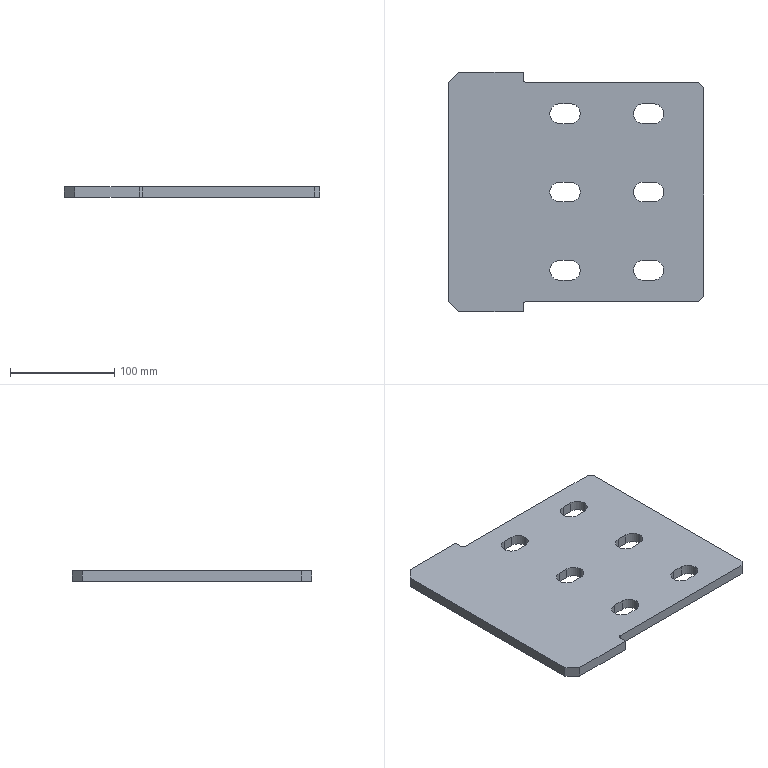Part | STEP file | 立柱腹Plate筋Plate-194×150-250 | 1 solid | 46 faces | box 245 x 230 x 10 mm | volume 499277 mm3 | plane 26 | cylinder 20 | commonest cylinder face diameters 19 x18 6 x2